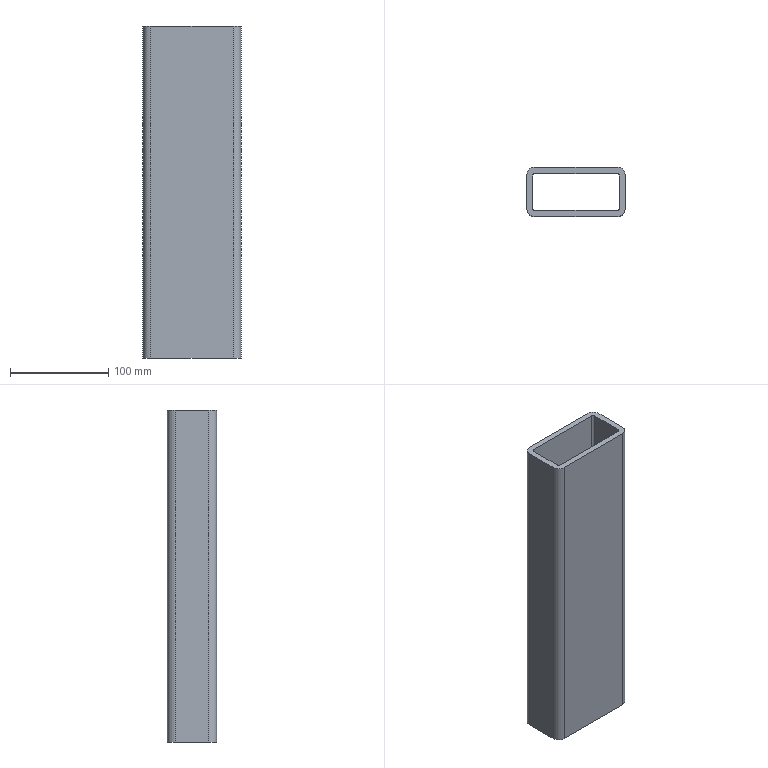Part | SolidWorks | features Extrusion 1, Shell 1 | 1 solid | 18 faces | box 100 x 50 x 337.5 mm | volume 541517 mm3 | plane 10 | cylinder 8 | commonest cylinder face diameters 4 x4 16 x4
STEP:
#1=CARTESIAN_POINT('',(-42.,25.,0.));
#2=VERTEX_POINT('',#1);
#3=CARTESIAN_POINT('',(-50.,17.,0.));
#4=VERTEX_POINT('',#3);
#5=CARTESIAN_POINT('',(-42.,17.,0.));
#6=DIRECTION('',(0.,0.,1.));
#7=DIRECTION('',(1.,0.,0.));
#8=AXIS2_PLACEMENT_3D('',#5,#6,#7);
#9=CIRCLE('',#8,8.);
#10=EDGE_CURVE('',#2,#4,#9,.T.);
#11=ORIENTED_EDGE('',*,*,#10,.T.);
#12=CARTESIAN_POINT('',(-50.,17.,337.5));
#13=VERTEX_POINT('',#12);
#14=CARTESIAN_POINT('',(-50.,17.,337.5));
#15=DIRECTION('',(0.,0.,-1.));
#16=VECTOR('',#15,1000.);
#17=LINE('',#14,#16);
#18=EDGE_CURVE('',#13,#4,#17,.T.);
#19=ORIENTED_EDGE('',*,*,#18,.F.);
#20=CARTESIAN_POINT('',(-42.,25.,337.5));
#21=VERTEX_POINT('',#20);
#22=CARTESIAN_POINT('',(-42.,17.,337.5));
#23=DIRECTION('',(0.,0.,1.));
#24=DIRECTION('',(1.,0.,0.));
#25=AXIS2_PLACEMENT_3D('',#22,#23,#24);
#26=CIRCLE('',#25,8.);
#27=EDGE_CURVE('',#21,#13,#26,.T.);
#28=ORIENTED_EDGE('',*,*,#27,.F.);
#29=CARTESIAN_POINT('',(-42.,25.,337.5));
#30=DIRECTION('',(0.,0.,-1.));
#31=VECTOR('',#30,1000.);
#32=LINE('',#29,#31);
#33=EDGE_CURVE('',#21,#2,#32,.T.);
#34=ORIENTED_EDGE('',*,*,#33,.T.);
#35=EDGE_LOOP('',(#11,#19,#28,#34));
#36=FACE_OUTER_BOUND('',#35,.T.);
#37=CARTESIAN_POINT('',(-42.,17.,337.5));
#38=DIRECTION('',(0.,0.,-1.));
#39=DIRECTION('',(-1.,0.,0.));
#40=AXIS2_PLACEMENT_3D('',#37,#38,#39);
#41=CYLINDRICAL_SURFACE('',#40,8.);
#42=ADVANCED_FACE('',(#36),#41,.T.);
#43=CARTESIAN_POINT('',(-50.,-17.,0.));
#44=VERTEX_POINT('',#43);
#45=CARTESIAN_POINT('',(-50.,17.,0.));
#46=DIRECTION('',(0.,-1.,0.));
#47=VECTOR('',#46,1000.);
#48=LINE('',#45,#47);
#49=EDGE_CURVE('',#4,#44,#48,.T.);
#50=ORIENTED_EDGE('',*,*,#49,.T.);
#51=CARTESIAN_POINT('',(-50.,-17.,337.5));
#52=VERTEX_POINT('',#51);
#53=CARTESIAN_POINT('',(-50.,-17.,337.5));
#54=DIRECTION('',(0.,0.,-1.));
#55=VECTOR('',#54,1000.);
#56=LINE('',#53,#55);
#57=EDGE_CURVE('',#52,#44,#56,.T.);
#58=ORIENTED_EDGE('',*,*,#57,.F.);
#59=CARTESIAN_POINT('',(-50.,17.,337.5));
#60=DIRECTION('',(0.,-1.,0.));
#61=VECTOR('',#60,1000.);
#62=LINE('',#59,#61);
#63=EDGE_CURVE('',#13,#52,#62,.T.);
#64=ORIENTED_EDGE('',*,*,#63,.F.);
#65=ORIENTED_EDGE('',*,*,#18,.T.);
#66=EDGE_LOOP('',(#50,#58,#64,#65));
#67=FACE_OUTER_BOUND('',#66,.T.);
#68=CARTESIAN_POINT('',(-50.,17.,337.5));
#69=DIRECTION('',(1.,0.,0.));
#70=DIRECTION('',(0.,1.,0.));
#71=AXIS2_PLACEMENT_3D('',#68,#69,#70);
#72=PLANE('',#71);
#73=ADVANCED_FACE('',(#67),#72,.F.);
#74=CARTESIAN_POINT('',(-42.,-25.,0.));
#75=VERTEX_POINT('',#74);
#76=CARTESIAN_POINT('',(-42.,-17.,0.));
#77=DIRECTION('',(0.,0.,-1.));
#78=DIRECTION('',(-1.,0.,0.));
#79=AXIS2_PLACEMENT_3D('',#76,#77,#78);
#80=CIRCLE('',#79,8.);
#81=EDGE_CURVE('',#75,#44,#80,.T.);
#82=ORIENTED_EDGE('',*,*,#81,.F.);
#83=CARTESIAN_POINT('',(-42.,-25.,337.5));
#84=VERTEX_POINT('',#83);
#85=CARTESIAN_POINT('',(-42.,-25.,337.5));
#86=DIRECTION('',(0.,0.,-1.));
#87=VECTOR('',#86,1000.);
#88=LINE('',#85,#87);
#89=EDGE_CURVE('',#84,#75,#88,.T.);
#90=ORIENTED_EDGE('',*,*,#89,.F.);
#91=CARTESIAN_POINT('',(-42.,-17.,337.5));
#92=DIRECTION('',(0.,0.,-1.));
#93=DIRECTION('',(-1.,0.,0.));
#94=AXIS2_PLACEMENT_3D('',#91,#92,#93);
#95=CIRCLE('',#94,8.);
#96=EDGE_CURVE('',#84,#52,#95,.T.);
#97=ORIENTED_EDGE('',*,*,#96,.T.);
#98=ORIENTED_EDGE('',*,*,#57,.T.);
#99=EDGE_LOOP('',(#82,#90,#97,#98));
#100=FACE_OUTER_BOUND('',#99,.T.);
#101=CARTESIAN_POINT('',(-42.,-17.,337.5));
#102=DIRECTION('',(0.,0.,-1.));
#103=DIRECTION('',(-1.,0.,0.));
#104=AXIS2_PLACEMENT_3D('',#101,#102,#103);
#105=CYLINDRICAL_SURFACE('',#104,8.);
#106=ADVANCED_FACE('',(#100),#105,.T.);
#107=CARTESIAN_POINT('',(42.,-25.,0.));
#108=VERTEX_POINT('',#107);
#109=CARTESIAN_POINT('',(42.,-25.,0.));
#110=DIRECTION('',(-1.,0.,0.));
#111=VECTOR('',#110,1000.);
#112=LINE('',#109,#111);
#113=EDGE_CURVE('',#108,#75,#112,.T.);
#114=ORIENTED_EDGE('',*,*,#113,.F.);
#115=CARTESIAN_POINT('',(42.,-25.,337.5));
#116=VERTEX_POINT('',#115);
#117=CARTESIAN_POINT('',(42.,-25.,337.5));
#118=DIRECTION('',(0.,0.,-1.));
#119=VECTOR('',#118,1000.);
#120=LINE('',#117,#119);
#121=EDGE_CURVE('',#116,#108,#120,.T.);
#122=ORIENTED_EDGE('',*,*,#121,.F.);
#123=CARTESIAN_POINT('',(42.,-25.,337.5));
#124=DIRECTION('',(-1.,0.,0.));
#125=VECTOR('',#124,1000.);
#126=LINE('',#123,#125);
#127=EDGE_CURVE('',#116,#84,#126,.T.);
#128=ORIENTED_EDGE('',*,*,#127,.T.);
#129=ORIENTED_EDGE('',*,*,#89,.T.);
#130=EDGE_LOOP('',(#114,#122,#128,#129));
#131=FACE_OUTER_BOUND('',#130,.T.);
#132=CARTESIAN_POINT('',(42.,-25.,337.5));
#133=DIRECTION('',(0.,-1.,0.));
#134=DIRECTION('',(1.,0.,0.));
#135=AXIS2_PLACEMENT_3D('',#132,#133,#134);
#136=PLANE('',#135);
#137=ADVANCED_FACE('',(#131),#136,.T.);
#138=CARTESIAN_POINT('',(50.,-17.,0.));
#139=VERTEX_POINT('',#138);
#140=CARTESIAN_POINT('',(42.,-17.,0.));
#141=DIRECTION('',(0.,0.,-1.));
#142=DIRECTION('',(-1.,0.,0.));
#143=AXIS2_PLACEMENT_3D('',#140,#141,#142);
#144=CIRCLE('',#143,8.);
#145=EDGE_CURVE('',#139,#108,#144,.T.);
#146=ORIENTED_EDGE('',*,*,#145,.F.);
#147=CARTESIAN_POINT('',(50.,-17.,337.5));
#148=VERTEX_POINT('',#147);
#149=CARTESIAN_POINT('',(50.,-17.,337.5));
#150=DIRECTION('',(0.,0.,-1.));
#151=VECTOR('',#150,1000.);
#152=LINE('',#149,#151);
#153=EDGE_CURVE('',#148,#139,#152,.T.);
#154=ORIENTED_EDGE('',*,*,#153,.F.);
#155=CARTESIAN_POINT('',(42.,-17.,337.5));
#156=DIRECTION('',(0.,0.,-1.));
#157=DIRECTION('',(-1.,0.,0.));
#158=AXIS2_PLACEMENT_3D('',#155,#156,#157);
#159=CIRCLE('',#158,8.);
#160=EDGE_CURVE('',#148,#116,#159,.T.);
#161=ORIENTED_EDGE('',*,*,#160,.T.);
#162=ORIENTED_EDGE('',*,*,#121,.T.);
#163=EDGE_LOOP('',(#146,#154,#161,#162));
#164=FACE_OUTER_BOUND('',#163,.T.);
#165=CARTESIAN_POINT('',(42.,-17.,337.5));
#166=DIRECTION('',(0.,0.,-1.));
#167=DIRECTION('',(-1.,0.,0.));
#168=AXIS2_PLACEMENT_3D('',#165,#166,#167);
#169=CYLINDRICAL_SURFACE('',#168,8.);
#170=ADVANCED_FACE('',(#164),#169,.T.);
#171=CARTESIAN_POINT('',(50.,17.,0.));
#172=VERTEX_POINT('',#171);
#173=CARTESIAN_POINT('',(50.,17.,0.));
#174=DIRECTION('',(0.,-1.,0.));
#175=VECTOR('',#174,1000.);
#176=LINE('',#173,#175);
#177=EDGE_CURVE('',#172,#139,#176,.T.);
#178=ORIENTED_EDGE('',*,*,#177,.F.);
#179=CARTESIAN_POINT('',(50.,17.,337.5));
#180=VERTEX_POINT('',#179);
#181=CARTESIAN_POINT('',(50.,17.,337.5));
#182=DIRECTION('',(0.,0.,-1.));
#183=VECTOR('',#182,1000.);
#184=LINE('',#181,#183);
#185=EDGE_CURVE('',#180,#172,#184,.T.);
#186=ORIENTED_EDGE('',*,*,#185,.F.);
#187=CARTESIAN_POINT('',(50.,17.,337.5));
#188=DIRECTION('',(0.,-1.,0.));
#189=VECTOR('',#188,1000.);
#190=LINE('',#187,#189);
#191=EDGE_CURVE('',#180,#148,#190,.T.);
#192=ORIENTED_EDGE('',*,*,#191,.T.);
#193=ORIENTED_EDGE('',*,*,#153,.T.);
#194=EDGE_LOOP('',(#178,#186,#192,#193));
#195=FACE_OUTER_BOUND('',#194,.T.);
#196=CARTESIAN_POINT('',(50.,17.,337.5));
#197=DIRECTION('',(1.,0.,0.));
#198=DIRECTION('',(0.,1.,0.));
#199=AXIS2_PLACEMENT_3D('',#196,#197,#198);
#200=PLANE('',#199);
#201=ADVANCED_FACE('',(#195),#200,.T.);
#202=CARTESIAN_POINT('',(42.,25.,0.));
#203=VERTEX_POINT('',#202);
#204=CARTESIAN_POINT('',(42.,17.,0.));
#205=DIRECTION('',(0.,0.,-1.));
#206=DIRECTION('',(-1.,0.,0.));
#207=AXIS2_PLACEMENT_3D('',#204,#205,#206);
#208=CIRCLE('',#207,8.);
#209=EDGE_CURVE('',#203,#172,#208,.T.);
#210=ORIENTED_EDGE('',*,*,#209,.F.);
#211=CARTESIAN_POINT('',(42.,25.,337.5));
#212=VERTEX_POINT('',#211);
#213=CARTESIAN_POINT('',(42.,25.,337.5));
#214=DIRECTION('',(0.,0.,-1.));
#215=VECTOR('',#214,1000.);
#216=LINE('',#213,#215);
#217=EDGE_CURVE('',#212,#203,#216,.T.);
#218=ORIENTED_EDGE('',*,*,#217,.F.);
#219=CARTESIAN_POINT('',(42.,17.,337.5));
#220=DIRECTION('',(0.,0.,-1.));
#221=DIRECTION('',(-1.,0.,0.));
#222=AXIS2_PLACEMENT_3D('',#219,#220,#221);
#223=CIRCLE('',#222,8.);
#224=EDGE_CURVE('',#212,#180,#223,.T.);
#225=ORIENTED_EDGE('',*,*,#224,.T.);
#226=ORIENTED_EDGE('',*,*,#185,.T.);
#227=EDGE_LOOP('',(#210,#218,#225,#226));
#228=FACE_OUTER_BOUND('',#227,.T.);
#229=CARTESIAN_POINT('',(42.,17.,337.5));
#230=DIRECTION('',(0.,0.,-1.));
#231=DIRECTION('',(-1.,0.,0.));
#232=AXIS2_PLACEMENT_3D('',#229,#230,#231);
#233=CYLINDRICAL_SURFACE('',#232,8.);
#234=ADVANCED_FACE('',(#228),#233,.T.);
#235=CARTESIAN_POINT('',(42.,25.,0.));
#236=DIRECTION('',(-1.,0.,0.));
#237=VECTOR('',#236,1000.);
#238=LINE('',#235,#237);
#239=EDGE_CURVE('',#203,#2,#238,.T.);
#240=ORIENTED_EDGE('',*,*,#239,.T.);
#241=ORIENTED_EDGE('',*,*,#33,.F.);
#242=CARTESIAN_POINT('',(42.,25.,337.5));
#243=DIRECTION('',(-1.,0.,0.));
#244=VECTOR('',#243,1000.);
#245=LINE('',#242,#244);
#246=EDGE_CURVE('',#212,#21,#245,.T.);
#247=ORIENTED_EDGE('',*,*,#246,.F.);
#248=ORIENTED_EDGE('',*,*,#217,.T.);
#249=EDGE_LOOP('',(#240,#241,#247,#248));
#250=FACE_OUTER_BOUND('',#249,.T.);
#251=CARTESIAN_POINT('',(42.,25.,337.5));
#252=DIRECTION('',(0.,-1.,0.));
#253=DIRECTION('',(1.,0.,0.));
#254=AXIS2_PLACEMENT_3D('',#251,#252,#253);
#255=PLANE('',#254);
#256=ADVANCED_FACE('',(#250),#255,.F.);
#257=CARTESIAN_POINT('',(-42.,19.,337.5));
#258=VERTEX_POINT('',#257);
#259=CARTESIAN_POINT('',(-44.,17.,337.5));
#260=VERTEX_POINT('',#259);
#261=CARTESIAN_POINT('',(-42.,17.,337.5));
#262=DIRECTION('',(0.,0.,1.));
#263=DIRECTION('',(1.,0.,0.));
#264=AXIS2_PLACEMENT_3D('',#261,#262,#263);
#265=CIRCLE('',#264,2.);
#266=EDGE_CURVE('',#258,#260,#265,.T.);
#267=ORIENTED_EDGE('',*,*,#266,.F.);
#268=CARTESIAN_POINT('',(42.,19.,337.5));
#269=VERTEX_POINT('',#268);
#270=CARTESIAN_POINT('',(42.,19.,337.5));
#271=DIRECTION('',(-1.,0.,0.));
#272=VECTOR('',#271,1000.);
#273=LINE('',#270,#272);
#274=EDGE_CURVE('',#269,#258,#273,.T.);
#275=ORIENTED_EDGE('',*,*,#274,.F.);
#276=CARTESIAN_POINT('',(44.,17.,337.5));
#277=VERTEX_POINT('',#276);
#278=CARTESIAN_POINT('',(42.,17.,337.5));
#279=DIRECTION('',(0.,0.,-1.));
#280=DIRECTION('',(1.,0.,0.));
#281=AXIS2_PLACEMENT_3D('',#278,#279,#280);
#282=CIRCLE('',#281,2.);
#283=EDGE_CURVE('',#269,#277,#282,.T.);
#284=ORIENTED_EDGE('',*,*,#283,.T.);
#285=CARTESIAN_POINT('',(44.,-17.,337.5));
#286=VERTEX_POINT('',#285);
#287=CARTESIAN_POINT('',(44.,17.,337.5));
#288=DIRECTION('',(0.,-1.,0.));
#289=VECTOR('',#288,1000.);
#290=LINE('',#287,#289);
#291=EDGE_CURVE('',#277,#286,#290,.T.);
#292=ORIENTED_EDGE('',*,*,#291,.T.);
#293=CARTESIAN_POINT('',(42.,-19.,337.5));
#294=VERTEX_POINT('',#293);
#295=CARTESIAN_POINT('',(42.,-17.,337.5));
#296=DIRECTION('',(0.,0.,-1.));
#297=DIRECTION('',(1.,0.,0.));
#298=AXIS2_PLACEMENT_3D('',#295,#296,#297);
#299=CIRCLE('',#298,2.);
#300=EDGE_CURVE('',#286,#294,#299,.T.);
#301=ORIENTED_EDGE('',*,*,#300,.T.);
#302=CARTESIAN_POINT('',(-42.,-19.,337.5));
#303=VERTEX_POINT('',#302);
#304=CARTESIAN_POINT('',(42.,-19.,337.5));
#305=DIRECTION('',(-1.,0.,0.));
#306=VECTOR('',#305,1000.);
#307=LINE('',#304,#306);
#308=EDGE_CURVE('',#294,#303,#307,.T.);
#309=ORIENTED_EDGE('',*,*,#308,.T.);
#310=CARTESIAN_POINT('',(-44.,-17.,337.5));
#311=VERTEX_POINT('',#310);
#312=CARTESIAN_POINT('',(-42.,-17.,337.5));
#313=DIRECTION('',(0.,0.,-1.));
#314=DIRECTION('',(1.,0.,0.));
#315=AXIS2_PLACEMENT_3D('',#312,#313,#314);
#316=CIRCLE('',#315,2.);
#317=EDGE_CURVE('',#303,#311,#316,.T.);
#318=ORIENTED_EDGE('',*,*,#317,.T.);
#319=CARTESIAN_POINT('',(-44.,17.,337.5));
#320=DIRECTION('',(0.,-1.,0.));
#321=VECTOR('',#320,1000.);
#322=LINE('',#319,#321);
#323=EDGE_CURVE('',#260,#311,#322,.T.);
#324=ORIENTED_EDGE('',*,*,#323,.F.);
#325=EDGE_LOOP('',(#267,#275,#284,#292,#301,#309,#318,#324));
#326=FACE_BOUND('',#325,.T.);
#327=ORIENTED_EDGE('',*,*,#27,.T.);
#328=ORIENTED_EDGE('',*,*,#63,.T.);
#329=ORIENTED_EDGE('',*,*,#96,.F.);
#330=ORIENTED_EDGE('',*,*,#127,.F.);
#331=ORIENTED_EDGE('',*,*,#160,.F.);
#332=ORIENTED_EDGE('',*,*,#191,.F.);
#333=ORIENTED_EDGE('',*,*,#224,.F.);
#334=ORIENTED_EDGE('',*,*,#246,.T.);
#335=EDGE_LOOP('',(#327,#328,#329,#330,#331,#332,#333,#334));
#336=FACE_OUTER_BOUND('',#335,.T.);
#337=CARTESIAN_POINT('',(-42.,17.,337.5));
#338=DIRECTION('',(0.,0.,1.));
#339=DIRECTION('',(1.,0.,0.));
#340=AXIS2_PLACEMENT_3D('',#337,#338,#339);
#341=PLANE('',#340);
#342=ADVANCED_FACE('',(#326,#336),#341,.T.);
#343=CARTESIAN_POINT('',(42.,19.,0.));
#344=VERTEX_POINT('',#343);
#345=CARTESIAN_POINT('',(-42.,19.,0.));
#346=VERTEX_POINT('',#345);
#347=CARTESIAN_POINT('',(42.,19.,0.));
#348=DIRECTION('',(-1.,0.,0.));
#349=VECTOR('',#348,1000.);
#350=LINE('',#347,#349);
#351=EDGE_CURVE('',#344,#346,#350,.T.);
#352=ORIENTED_EDGE('',*,*,#351,.T.);
#353=CARTESIAN_POINT('',(-44.,17.,0.));
#354=VERTEX_POINT('',#353);
#355=CARTESIAN_POINT('',(-42.,17.,0.));
#356=DIRECTION('',(0.,0.,1.));
#357=DIRECTION('',(1.,0.,0.));
#358=AXIS2_PLACEMENT_3D('',#355,#356,#357);
#359=CIRCLE('',#358,2.);
#360=EDGE_CURVE('',#346,#354,#359,.T.);
#361=ORIENTED_EDGE('',*,*,#360,.T.);
#362=CARTESIAN_POINT('',(-44.,-17.,0.));
#363=VERTEX_POINT('',#362);
#364=CARTESIAN_POINT('',(-44.,17.,0.));
#365=DIRECTION('',(0.,-1.,0.));
#366=VECTOR('',#365,1000.);
#367=LINE('',#364,#366);
#368=EDGE_CURVE('',#354,#363,#367,.T.);
#369=ORIENTED_EDGE('',*,*,#368,.T.);
#370=CARTESIAN_POINT('',(-42.,-19.,0.));
#371=VERTEX_POINT('',#370);
#372=CARTESIAN_POINT('',(-42.,-17.,0.));
#373=DIRECTION('',(0.,0.,-1.));
#374=DIRECTION('',(1.,0.,0.));
#375=AXIS2_PLACEMENT_3D('',#372,#373,#374);
#376=CIRCLE('',#375,2.);
#377=EDGE_CURVE('',#371,#363,#376,.T.);
#378=ORIENTED_EDGE('',*,*,#377,.F.);
#379=CARTESIAN_POINT('',(42.,-19.,0.));
#380=VERTEX_POINT('',#379);
#381=CARTESIAN_POINT('',(42.,-19.,0.));
#382=DIRECTION('',(-1.,0.,0.));
#383=VECTOR('',#382,1000.);
#384=LINE('',#381,#383);
#385=EDGE_CURVE('',#380,#371,#384,.T.);
#386=ORIENTED_EDGE('',*,*,#385,.F.);
#387=CARTESIAN_POINT('',(44.,-17.,0.));
#388=VERTEX_POINT('',#387);
#389=CARTESIAN_POINT('',(42.,-17.,0.));
#390=DIRECTION('',(0.,0.,-1.));
#391=DIRECTION('',(1.,0.,0.));
#392=AXIS2_PLACEMENT_3D('',#389,#390,#391);
#393=CIRCLE('',#392,2.);
#394=EDGE_CURVE('',#388,#380,#393,.T.);
#395=ORIENTED_EDGE('',*,*,#394,.F.);
#396=CARTESIAN_POINT('',(44.,17.,0.));
#397=VERTEX_POINT('',#396);
#398=CARTESIAN_POINT('',(44.,17.,0.));
#399=DIRECTION('',(0.,-1.,0.));
#400=VECTOR('',#399,1000.);
#401=LINE('',#398,#400);
#402=EDGE_CURVE('',#397,#388,#401,.T.);
#403=ORIENTED_EDGE('',*,*,#402,.F.);
#404=CARTESIAN_POINT('',(42.,17.,0.));
#405=DIRECTION('',(0.,0.,-1.));
#406=DIRECTION('',(1.,0.,0.));
#407=AXIS2_PLACEMENT_3D('',#404,#405,#406);
#408=CIRCLE('',#407,2.);
#409=EDGE_CURVE('',#344,#397,#408,.T.);
#410=ORIENTED_EDGE('',*,*,#409,.F.);
#411=EDGE_LOOP('',(#352,#361,#369,#378,#386,#395,#403,#410));
#412=FACE_BOUND('',#411,.T.);
#413=ORIENTED_EDGE('',*,*,#10,.F.);
#414=ORIENTED_EDGE('',*,*,#239,.F.);
#415=ORIENTED_EDGE('',*,*,#209,.T.);
#416=ORIENTED_EDGE('',*,*,#177,.T.);
#417=ORIENTED_EDGE('',*,*,#145,.T.);
#418=ORIENTED_EDGE('',*,*,#113,.T.);
#419=ORIENTED_EDGE('',*,*,#81,.T.);
#420=ORIENTED_EDGE('',*,*,#49,.F.);
#421=EDGE_LOOP('',(#413,#414,#415,#416,#417,#418,#419,#420));
#422=FACE_OUTER_BOUND('',#421,.T.);
#423=CARTESIAN_POINT('',(-42.,17.,0.));
#424=DIRECTION('',(0.,0.,1.));
#425=DIRECTION('',(1.,0.,0.));
#426=AXIS2_PLACEMENT_3D('',#423,#424,#425);
#427=PLANE('',#426);
#428=ADVANCED_FACE('',(#412,#422),#427,.F.);
#429=ORIENTED_EDGE('',*,*,#360,.F.);
#430=CARTESIAN_POINT('',(-42.,19.,337.5));
#431=DIRECTION('',(0.,0.,-1.));
#432=VECTOR('',#431,1000.);
#433=LINE('',#430,#432);
#434=EDGE_CURVE('',#258,#346,#433,.T.);
#435=ORIENTED_EDGE('',*,*,#434,.F.);
#436=ORIENTED_EDGE('',*,*,#266,.T.);
#437=CARTESIAN_POINT('',(-44.,17.,337.5));
#438=DIRECTION('',(0.,0.,-1.));
#439=VECTOR('',#438,1000.);
#440=LINE('',#437,#439);
#441=EDGE_CURVE('',#260,#354,#440,.T.);
#442=ORIENTED_EDGE('',*,*,#441,.T.);
#443=EDGE_LOOP('',(#429,#435,#436,#442));
#444=FACE_OUTER_BOUND('',#443,.T.);
#445=CARTESIAN_POINT('',(-42.,17.,337.5));
#446=DIRECTION('',(0.,0.,-1.));
#447=DIRECTION('',(-1.,0.,0.));
#448=AXIS2_PLACEMENT_3D('',#445,#446,#447);
#449=CYLINDRICAL_SURFACE('',#448,2.);
#450=ADVANCED_FACE('',(#444),#449,.F.);
#451=ORIENTED_EDGE('',*,*,#368,.F.);
#452=ORIENTED_EDGE('',*,*,#441,.F.);
#453=ORIENTED_EDGE('',*,*,#323,.T.);
#454=CARTESIAN_POINT('',(-44.,-17.,337.5));
#455=DIRECTION('',(0.,0.,-1.));
#456=VECTOR('',#455,1000.);
#457=LINE('',#454,#456);
#458=EDGE_CURVE('',#311,#363,#457,.T.);
#459=ORIENTED_EDGE('',*,*,#458,.T.);
#460=EDGE_LOOP('',(#451,#452,#453,#459));
#461=FACE_OUTER_BOUND('',#460,.T.);
#462=CARTESIAN_POINT('',(-44.,17.,337.5));
#463=DIRECTION('',(1.,0.,0.));
#464=DIRECTION('',(0.,1.,0.));
#465=AXIS2_PLACEMENT_3D('',#462,#463,#464);
#466=PLANE('',#465);
#467=ADVANCED_FACE('',(#461),#466,.T.);
#468=ORIENTED_EDGE('',*,*,#377,.T.);
#469=ORIENTED_EDGE('',*,*,#458,.F.);
#470=ORIENTED_EDGE('',*,*,#317,.F.);
#471=CARTESIAN_POINT('',(-42.,-19.,337.5));
#472=DIRECTION('',(0.,0.,-1.));
#473=VECTOR('',#472,1000.);
#474=LINE('',#471,#473);
#475=EDGE_CURVE('',#303,#371,#474,.T.);
#476=ORIENTED_EDGE('',*,*,#475,.T.);
#477=EDGE_LOOP('',(#468,#469,#470,#476));
#478=FACE_OUTER_BOUND('',#477,.T.);
#479=CARTESIAN_POINT('',(-42.,-17.,337.5));
#480=DIRECTION('',(0.,0.,-1.));
#481=DIRECTION('',(-1.,0.,0.));
#482=AXIS2_PLACEMENT_3D('',#479,#480,#481);
#483=CYLINDRICAL_SURFACE('',#482,2.);
#484=ADVANCED_FACE('',(#478),#483,.F.);
#485=ORIENTED_EDGE('',*,*,#385,.T.);
#486=ORIENTED_EDGE('',*,*,#475,.F.);
#487=ORIENTED_EDGE('',*,*,#308,.F.);
#488=CARTESIAN_POINT('',(42.,-19.,337.5));
#489=DIRECTION('',(0.,0.,-1.));
#490=VECTOR('',#489,1000.);
#491=LINE('',#488,#490);
#492=EDGE_CURVE('',#294,#380,#491,.T.);
#493=ORIENTED_EDGE('',*,*,#492,.T.);
#494=EDGE_LOOP('',(#485,#486,#487,#493));
#495=FACE_OUTER_BOUND('',#494,.T.);
#496=CARTESIAN_POINT('',(42.,-19.,337.5));
#497=DIRECTION('',(0.,-1.,0.));
#498=DIRECTION('',(1.,0.,0.));
#499=AXIS2_PLACEMENT_3D('',#496,#497,#498);
#500=PLANE('',#499);
#501=ADVANCED_FACE('',(#495),#500,.F.);
#502=ORIENTED_EDGE('',*,*,#394,.T.);
#503=ORIENTED_EDGE('',*,*,#492,.F.);
#504=ORIENTED_EDGE('',*,*,#300,.F.);
#505=CARTESIAN_POINT('',(44.,-17.,337.5));
#506=DIRECTION('',(0.,0.,-1.));
#507=VECTOR('',#506,1000.);
#508=LINE('',#505,#507);
#509=EDGE_CURVE('',#286,#388,#508,.T.);
#510=ORIENTED_EDGE('',*,*,#509,.T.);
#511=EDGE_LOOP('',(#502,#503,#504,#510));
#512=FACE_OUTER_BOUND('',#511,.T.);
#513=CARTESIAN_POINT('',(42.,-17.,337.5));
#514=DIRECTION('',(0.,0.,-1.));
#515=DIRECTION('',(-1.,0.,0.));
#516=AXIS2_PLACEMENT_3D('',#513,#514,#515);
#517=CYLINDRICAL_SURFACE('',#516,2.);
#518=ADVANCED_FACE('',(#512),#517,.F.);
#519=ORIENTED_EDGE('',*,*,#402,.T.);
#520=ORIENTED_EDGE('',*,*,#509,.F.);
#521=ORIENTED_EDGE('',*,*,#291,.F.);
#522=CARTESIAN_POINT('',(44.,17.,337.5));
#523=DIRECTION('',(0.,0.,-1.));
#524=VECTOR('',#523,1000.);
#525=LINE('',#522,#524);
#526=EDGE_CURVE('',#277,#397,#525,.T.);
#527=ORIENTED_EDGE('',*,*,#526,.T.);
#528=EDGE_LOOP('',(#519,#520,#521,#527));
#529=FACE_OUTER_BOUND('',#528,.T.);
#530=CARTESIAN_POINT('',(44.,17.,337.5));
#531=DIRECTION('',(1.,0.,0.));
#532=DIRECTION('',(0.,1.,0.));
#533=AXIS2_PLACEMENT_3D('',#530,#531,#532);
#534=PLANE('',#533);
#535=ADVANCED_FACE('',(#529),#534,.F.);
#536=ORIENTED_EDGE('',*,*,#409,.T.);
#537=ORIENTED_EDGE('',*,*,#526,.F.);
#538=ORIENTED_EDGE('',*,*,#283,.F.);
#539=CARTESIAN_POINT('',(42.,19.,337.5));
#540=DIRECTION('',(0.,0.,-1.));
#541=VECTOR('',#540,1000.);
#542=LINE('',#539,#541);
#543=EDGE_CURVE('',#269,#344,#542,.T.);
#544=ORIENTED_EDGE('',*,*,#543,.T.);
#545=EDGE_LOOP('',(#536,#537,#538,#544));
#546=FACE_OUTER_BOUND('',#545,.T.);
#547=CARTESIAN_POINT('',(42.,17.,337.5));
#548=DIRECTION('',(0.,0.,-1.));
#549=DIRECTION('',(-1.,0.,0.));
#550=AXIS2_PLACEMENT_3D('',#547,#548,#549);
#551=CYLINDRICAL_SURFACE('',#550,2.);
#552=ADVANCED_FACE('',(#546),#551,.F.);
#553=ORIENTED_EDGE('',*,*,#351,.F.);
#554=ORIENTED_EDGE('',*,*,#543,.F.);
#555=ORIENTED_EDGE('',*,*,#274,.T.);
#556=ORIENTED_EDGE('',*,*,#434,.T.);
#557=EDGE_LOOP('',(#553,#554,#555,#556));
#558=FACE_OUTER_BOUND('',#557,.T.);
#559=CARTESIAN_POINT('',(42.,19.,337.5));
#560=DIRECTION('',(0.,-1.,0.));
#561=DIRECTION('',(1.,0.,0.));
#562=AXIS2_PLACEMENT_3D('',#559,#560,#561);
#563=PLANE('',#562);
#564=ADVANCED_FACE('',(#558),#563,.T.);
#565=CLOSED_SHELL('',(#42,#73,#106,#137,#170,#201,#234,#256,#342,#428,#450,#467,#484,#501,#518,#535,#552,#564));
#566=MANIFOLD_SOLID_BREP('',#565);
#567=CARTESIAN_POINT('',(0.,0.,0.));
#568=DIRECTION('',(0.,0.,1.));
#569=DIRECTION('',(1.,0.,0.));
#570=AXIS2_PLACEMENT_3D('',#567,#568,#569);
#571=(LENGTH_UNIT()NAMED_UNIT(*)SI_UNIT(.MILLI.,.METRE.));
#572=UNCERTAINTY_MEASURE_WITH_UNIT(LENGTH_MEASURE(0.00001),#571,'','');
#573=(NAMED_UNIT(*)PLANE_ANGLE_UNIT()SI_UNIT($,.RADIAN.));
#574=(NAMED_UNIT(*)SI_UNIT($,.STERADIAN.)SOLID_ANGLE_UNIT());
#575=(GEOMETRIC_REPRESENTATION_CONTEXT(3)GLOBAL_UNCERTAINTY_ASSIGNED_CONTEXT((#572))GLOBAL_UNIT_ASSIGNED_CONTEXT((#571,#573,#574))REPRESENTATION_CONTEXT('',''));
#576=ADVANCED_BREP_SHAPE_REPRESENTATION('',(#566,#570),#575);